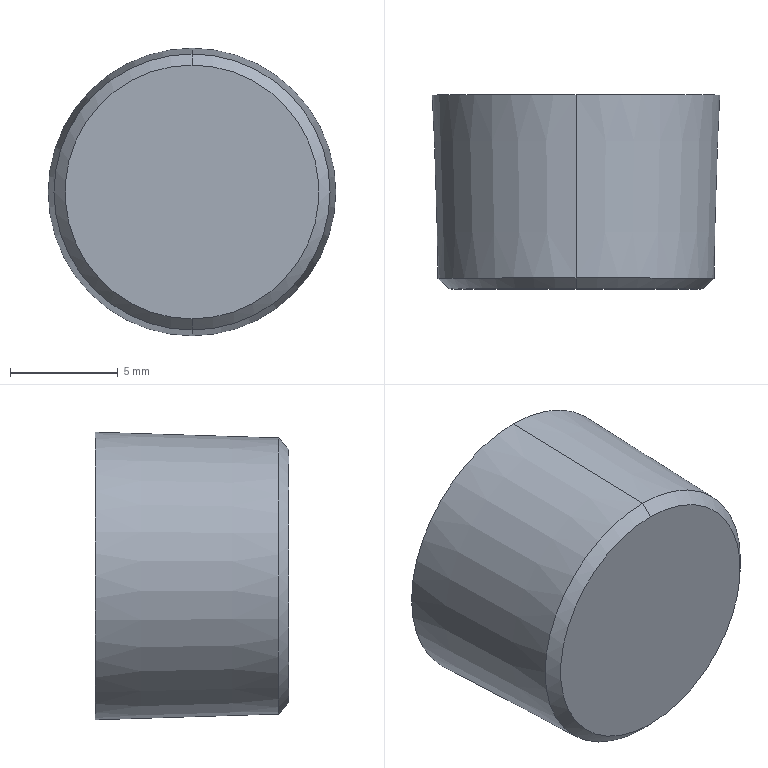Part | SolidWorks | features BaseBody 1 | 1 solid | 23 faces | box 13.344 x 9 x 13.344 mm | volume 1017 mm3 | plane 15 | cone 8
STEP:
#1=CARTESIAN_POINT('',(0.,0.4998,6.407));
#2=VERTEX_POINT('',#1);
#3=CARTESIAN_POINT('',(0.,0.4998,-6.407));
#4=VERTEX_POINT('',#3);
#5=CARTESIAN_POINT('',(0.,0.4998,0.));
#6=DIRECTION('',(0.,1.,0.));
#7=DIRECTION('',(0.,0.,1.));
#8=AXIS2_PLACEMENT_3D('',#5,#6,#7);
#9=CIRCLE('',#8,6.407);
#10=EDGE_CURVE('',#2,#4,#9,.T.);
#11=ORIENTED_EDGE('',*,*,#10,.T.);
#12=CARTESIAN_POINT('',(0.,9.,-6.672));
#13=VERTEX_POINT('',#12);
#14=CARTESIAN_POINT('',(0.,9.,-6.672));
#15=DIRECTION('',(0.,0.9995,-0.0312));
#16=VECTOR('',#15,1000.);
#17=LINE('',#14,#16);
#18=EDGE_CURVE('',#4,#13,#17,.T.);
#19=ORIENTED_EDGE('',*,*,#18,.T.);
#20=CARTESIAN_POINT('',(0.,9.,6.672));
#21=VERTEX_POINT('',#20);
#22=CARTESIAN_POINT('',(0.,9.,0.));
#23=DIRECTION('',(0.,-1.,0.));
#24=DIRECTION('',(0.,0.,1.));
#25=AXIS2_PLACEMENT_3D('',#22,#23,#24);
#26=CIRCLE('',#25,6.672);
#27=EDGE_CURVE('',#13,#21,#26,.T.);
#28=ORIENTED_EDGE('',*,*,#27,.T.);
#29=CARTESIAN_POINT('',(0.,9.,6.672));
#30=DIRECTION('',(0.,0.9995,0.0312));
#31=VECTOR('',#30,1000.);
#32=LINE('',#29,#31);
#33=EDGE_CURVE('',#2,#21,#32,.T.);
#34=ORIENTED_EDGE('',*,*,#33,.F.);
#35=EDGE_LOOP('',(#11,#19,#28,#34));
#36=FACE_OUTER_BOUND('',#35,.T.);
#37=CARTESIAN_POINT('',(0.,9.,0.));
#38=DIRECTION('',(0.,1.,0.));
#39=DIRECTION('',(0.,0.,1.));
#40=AXIS2_PLACEMENT_3D('',#37,#38,#39);
#41=CONICAL_SURFACE('',#40,6.672,0.03121);
#42=ADVANCED_FACE('',(#36),#41,.T.);
#43=CARTESIAN_POINT('',(0.,0.,5.891));
#44=VERTEX_POINT('',#43);
#45=CARTESIAN_POINT('',(0.,0.,-5.891));
#46=VERTEX_POINT('',#45);
#47=CARTESIAN_POINT('',(0.,0.,0.));
#48=DIRECTION('',(0.,1.,0.));
#49=DIRECTION('',(0.,0.,1.));
#50=AXIS2_PLACEMENT_3D('',#47,#48,#49);
#51=CIRCLE('',#50,5.891);
#52=EDGE_CURVE('',#44,#46,#51,.T.);
#53=ORIENTED_EDGE('',*,*,#52,.T.);
#54=CARTESIAN_POINT('',(0.,0.4998,-6.407));
#55=DIRECTION('',(0.,0.696,-0.7181));
#56=VECTOR('',#55,1000.);
#57=LINE('',#54,#56);
#58=EDGE_CURVE('',#46,#4,#57,.T.);
#59=ORIENTED_EDGE('',*,*,#58,.T.);
#60=ORIENTED_EDGE('',*,*,#10,.F.);
#61=CARTESIAN_POINT('',(0.,0.4998,6.407));
#62=DIRECTION('',(0.,0.696,0.7181));
#63=VECTOR('',#62,1000.);
#64=LINE('',#61,#63);
#65=EDGE_CURVE('',#44,#2,#64,.T.);
#66=ORIENTED_EDGE('',*,*,#65,.F.);
#67=EDGE_LOOP('',(#53,#59,#60,#66));
#68=FACE_OUTER_BOUND('',#67,.T.);
#69=CARTESIAN_POINT('',(0.,0.4998,0.));
#70=DIRECTION('',(0.,1.,0.));
#71=DIRECTION('',(0.,0.,1.));
#72=AXIS2_PLACEMENT_3D('',#69,#70,#71);
#73=CONICAL_SURFACE('',#72,6.407,0.801);
#74=ADVANCED_FACE('',(#68),#73,.T.);
#75=CARTESIAN_POINT('',(0.,8.293,-3.));
#76=VERTEX_POINT('',#75);
#77=CARTESIAN_POINT('',(-1.732,8.757,-3.));
#78=VERTEX_POINT('',#77);
#79=CARTESIAN_POINT('',(0.,8.293,-3.));
#80=CARTESIAN_POINT('',(-0.3013,8.293,-3.));
#81=CARTESIAN_POINT('',(-0.5974,8.339,-3.));
#82=CARTESIAN_POINT('',(-1.182,8.505,-3.));
#83=CARTESIAN_POINT('',(-1.461,8.621,-3.));
#84=CARTESIAN_POINT('',(-1.732,8.757,-3.));
#85=B_SPLINE_CURVE_WITH_KNOTS('',3,(#79,#80,#81,#82,#83,#84),.UNSPECIFIED.,.F.,.F.,(4,2,4),(0.001795,0.002687,0.003578),.UNSPECIFIED.);
#86=EDGE_CURVE('',#76,#78,#85,.T.);
#87=ORIENTED_EDGE('',*,*,#86,.F.);
#88=CARTESIAN_POINT('',(0.,9.,-3.707));
#89=VERTEX_POINT('',#88);
#90=CARTESIAN_POINT('',(0.,9.,-3.707));
#91=DIRECTION('',(0.,0.7071,-0.7071));
#92=VECTOR('',#91,1000.);
#93=LINE('',#90,#92);
#94=EDGE_CURVE('',#76,#89,#93,.T.);
#95=ORIENTED_EDGE('',*,*,#94,.T.);
#96=CARTESIAN_POINT('',(0.,9.,3.707));
#97=VERTEX_POINT('',#96);
#98=CARTESIAN_POINT('',(0.,9.,0.));
#99=DIRECTION('',(0.,1.,0.));
#100=DIRECTION('',(0.,0.,1.));
#101=AXIS2_PLACEMENT_3D('',#98,#99,#100);
#102=CIRCLE('',#101,3.707);
#103=EDGE_CURVE('',#89,#97,#102,.T.);
#104=ORIENTED_EDGE('',*,*,#103,.T.);
#105=CARTESIAN_POINT('',(0.,8.293,3.));
#106=VERTEX_POINT('',#105);
#107=CARTESIAN_POINT('',(0.,9.,3.707));
#108=DIRECTION('',(0.,0.7071,0.7071));
#109=VECTOR('',#108,1000.);
#110=LINE('',#107,#109);
#111=EDGE_CURVE('',#106,#97,#110,.T.);
#112=ORIENTED_EDGE('',*,*,#111,.F.);
#113=CARTESIAN_POINT('',(-1.732,8.757,3.));
#114=VERTEX_POINT('',#113);
#115=CARTESIAN_POINT('',(-1.732,8.757,3.));
#116=CARTESIAN_POINT('',(-1.46,8.621,3.));
#117=CARTESIAN_POINT('',(-1.183,8.506,3.));
#118=CARTESIAN_POINT('',(-0.7511,8.382,3.));
#119=CARTESIAN_POINT('',(-0.6047,8.35,3.));
#120=CARTESIAN_POINT('',(-0.3057,8.305,3.));
#121=CARTESIAN_POINT('',(-0.1517,8.293,3.));
#122=CARTESIAN_POINT('',(0.,8.293,3.));
#123=B_SPLINE_CURVE_WITH_KNOTS('',3,(#115,#116,#117,#118,#119,#120,#121,#122),.UNSPECIFIED.,.F.,.F.,(4,2,2,4),(0.,0.0008977,0.001347,0.001795),.UNSPECIFIED.);
#124=EDGE_CURVE('',#114,#106,#123,.T.);
#125=ORIENTED_EDGE('',*,*,#124,.F.);
#126=CARTESIAN_POINT('',(-3.464,8.757,-0.000000032));
#127=VERTEX_POINT('',#126);
#128=CARTESIAN_POINT('',(-3.464,8.757,-0.000000032));
#129=CARTESIAN_POINT('',(-3.329,8.622,0.2344));
#130=CARTESIAN_POINT('',(-3.19,8.507,0.4741));
#131=CARTESIAN_POINT('',(-2.975,8.383,0.8465));
#132=CARTESIAN_POINT('',(-2.902,8.351,0.9728));
#133=CARTESIAN_POINT('',(-2.754,8.305,1.231));
#134=CARTESIAN_POINT('',(-2.677,8.293,1.364));
#135=CARTESIAN_POINT('',(-2.45,8.292,1.756));
#136=CARTESIAN_POINT('',(-2.301,8.338,2.014));
#137=CARTESIAN_POINT('',(-2.008,8.504,2.521));
#138=CARTESIAN_POINT('',(-1.868,8.621,2.764));
#139=CARTESIAN_POINT('',(-1.732,8.757,3.));
#140=B_SPLINE_CURVE_WITH_KNOTS('',3,(#128,#129,#130,#131,#132,#133,#134,#135,#136,#137,#138,#139),.UNSPECIFIED.,.F.,.F.,(4,2,2,2,2,4),(0.,0.0008946,0.001342,0.001789,0.002684,0.003578),.UNSPECIFIED.);
#141=EDGE_CURVE('',#127,#114,#140,.T.);
#142=ORIENTED_EDGE('',*,*,#141,.F.);
#143=CARTESIAN_POINT('',(-1.732,8.757,-3.));
#144=CARTESIAN_POINT('',(-1.867,8.622,-2.766));
#145=CARTESIAN_POINT('',(-2.006,8.507,-2.526));
#146=CARTESIAN_POINT('',(-2.221,8.383,-2.154));
#147=CARTESIAN_POINT('',(-2.294,8.351,-2.027));
#148=CARTESIAN_POINT('',(-2.443,8.305,-1.769));
#149=CARTESIAN_POINT('',(-2.519,8.293,-1.636));
#150=CARTESIAN_POINT('',(-2.746,8.292,-1.244));
#151=CARTESIAN_POINT('',(-2.895,8.338,-0.9862));
#152=CARTESIAN_POINT('',(-3.188,8.504,-0.4785));
#153=CARTESIAN_POINT('',(-3.328,8.621,-0.2358));
#154=CARTESIAN_POINT('',(-3.464,8.757,-0.000000032));
#155=B_SPLINE_CURVE_WITH_KNOTS('',3,(#143,#144,#145,#146,#147,#148,#149,#150,#151,#152,#153,#154),.UNSPECIFIED.,.F.,.F.,(4,2,2,2,2,4),(0.,0.0008946,0.001342,0.001789,0.002684,0.003578),.UNSPECIFIED.);
#156=EDGE_CURVE('',#78,#127,#155,.T.);
#157=ORIENTED_EDGE('',*,*,#156,.F.);
#158=EDGE_LOOP('',(#87,#95,#104,#112,#125,#142,#157));
#159=FACE_OUTER_BOUND('',#158,.T.);
#160=CARTESIAN_POINT('',(0.,9.,0.));
#161=DIRECTION('',(0.,1.,0.));
#162=DIRECTION('',(0.,0.,1.));
#163=AXIS2_PLACEMENT_3D('',#160,#161,#162);
#164=CONICAL_SURFACE('',#163,3.707,0.7854);
#165=ADVANCED_FACE('',(#159),#164,.F.);
#166=CARTESIAN_POINT('',(1.831,3.063,0.));
#167=VERTEX_POINT('',#166);
#168=CARTESIAN_POINT('',(-1.831,3.063,0.));
#169=VERTEX_POINT('',#168);
#170=CARTESIAN_POINT('',(0.,3.063,0.));
#171=DIRECTION('',(0.,1.,0.));
#172=DIRECTION('',(-1.,0.,0.));
#173=AXIS2_PLACEMENT_3D('',#170,#171,#172);
#174=CIRCLE('',#173,1.831);
#175=EDGE_CURVE('',#167,#169,#174,.T.);
#176=ORIENTED_EDGE('',*,*,#175,.F.);
#177=CARTESIAN_POINT('',(3.464,3.5,0.));
#178=VERTEX_POINT('',#177);
#179=CARTESIAN_POINT('',(3.464,3.5,0.));
#180=DIRECTION('',(0.9659,0.2588,0.));
#181=VECTOR('',#180,1000.);
#182=LINE('',#179,#181);
#183=EDGE_CURVE('',#167,#178,#182,.T.);
#184=ORIENTED_EDGE('',*,*,#183,.T.);
#185=CARTESIAN_POINT('',(1.732,3.5,-3.));
#186=VERTEX_POINT('',#185);
#187=CARTESIAN_POINT('',(0.,3.5,0.));
#188=DIRECTION('',(0.,-1.,0.));
#189=DIRECTION('',(-1.,0.,0.));
#190=AXIS2_PLACEMENT_3D('',#187,#188,#189);
#191=CIRCLE('',#190,3.464);
#192=EDGE_CURVE('',#186,#178,#191,.T.);
#193=ORIENTED_EDGE('',*,*,#192,.F.);
#194=CARTESIAN_POINT('',(-1.732,3.5,-3.));
#195=VERTEX_POINT('',#194);
#196=CARTESIAN_POINT('',(0.,3.5,0.));
#197=DIRECTION('',(0.,-1.,0.));
#198=DIRECTION('',(-1.,0.,0.));
#199=AXIS2_PLACEMENT_3D('',#196,#197,#198);
#200=CIRCLE('',#199,3.464);
#201=EDGE_CURVE('',#195,#186,#200,.T.);
#202=ORIENTED_EDGE('',*,*,#201,.F.);
#203=CARTESIAN_POINT('',(-3.464,3.5,0.));
#204=VERTEX_POINT('',#203);
#205=CARTESIAN_POINT('',(0.,3.5,0.));
#206=DIRECTION('',(0.,-1.,0.));
#207=DIRECTION('',(-1.,0.,0.));
#208=AXIS2_PLACEMENT_3D('',#205,#206,#207);
#209=CIRCLE('',#208,3.464);
#210=EDGE_CURVE('',#204,#195,#209,.T.);
#211=ORIENTED_EDGE('',*,*,#210,.F.);
#212=CARTESIAN_POINT('',(-3.464,3.5,0.));
#213=DIRECTION('',(-0.9659,0.2588,0.));
#214=VECTOR('',#213,1000.);
#215=LINE('',#212,#214);
#216=EDGE_CURVE('',#169,#204,#215,.T.);
#217=ORIENTED_EDGE('',*,*,#216,.F.);
#218=EDGE_LOOP('',(#176,#184,#193,#202,#211,#217));
#219=FACE_OUTER_BOUND('',#218,.T.);
#220=CARTESIAN_POINT('',(0.,3.5,0.));
#221=DIRECTION('',(0.,1.,0.));
#222=DIRECTION('',(-1.,0.,0.));
#223=AXIS2_PLACEMENT_3D('',#220,#221,#222);
#224=CONICAL_SURFACE('',#223,3.464,1.309);
#225=ADVANCED_FACE('',(#219),#224,.F.);
#226=ORIENTED_EDGE('',*,*,#18,.F.);
#227=CARTESIAN_POINT('',(0.,0.4998,0.));
#228=DIRECTION('',(0.,1.,0.));
#229=DIRECTION('',(0.,0.,1.));
#230=AXIS2_PLACEMENT_3D('',#227,#228,#229);
#231=CIRCLE('',#230,6.407);
#232=EDGE_CURVE('',#4,#2,#231,.T.);
#233=ORIENTED_EDGE('',*,*,#232,.T.);
#234=ORIENTED_EDGE('',*,*,#33,.T.);
#235=CARTESIAN_POINT('',(0.,9.,0.));
#236=DIRECTION('',(0.,-1.,0.));
#237=DIRECTION('',(0.,0.,1.));
#238=AXIS2_PLACEMENT_3D('',#235,#236,#237);
#239=CIRCLE('',#238,6.672);
#240=EDGE_CURVE('',#21,#13,#239,.T.);
#241=ORIENTED_EDGE('',*,*,#240,.T.);
#242=EDGE_LOOP('',(#226,#233,#234,#241));
#243=FACE_OUTER_BOUND('',#242,.T.);
#244=CARTESIAN_POINT('',(0.,9.,0.));
#245=DIRECTION('',(0.,1.,0.));
#246=DIRECTION('',(0.,0.,1.));
#247=AXIS2_PLACEMENT_3D('',#244,#245,#246);
#248=CONICAL_SURFACE('',#247,6.672,0.03121);
#249=ADVANCED_FACE('',(#243),#248,.T.);
#250=CARTESIAN_POINT('',(0.,9.,0.));
#251=DIRECTION('',(0.,1.,0.));
#252=DIRECTION('',(0.,0.,1.));
#253=AXIS2_PLACEMENT_3D('',#250,#251,#252);
#254=CIRCLE('',#253,3.707);
#255=EDGE_CURVE('',#97,#89,#254,.T.);
#256=ORIENTED_EDGE('',*,*,#255,.F.);
#257=ORIENTED_EDGE('',*,*,#103,.F.);
#258=EDGE_LOOP('',(#256,#257));
#259=FACE_BOUND('',#258,.T.);
#260=ORIENTED_EDGE('',*,*,#240,.F.);
#261=ORIENTED_EDGE('',*,*,#27,.F.);
#262=EDGE_LOOP('',(#260,#261));
#263=FACE_OUTER_BOUND('',#262,.T.);
#264=CARTESIAN_POINT('',(3.707,9.,0.));
#265=DIRECTION('',(0.,-1.,0.));
#266=DIRECTION('',(0.,0.,-1.));
#267=AXIS2_PLACEMENT_3D('',#264,#265,#266);
#268=PLANE('',#267);
#269=ADVANCED_FACE('',(#259,#263),#268,.F.);
#270=ORIENTED_EDGE('',*,*,#58,.F.);
#271=CARTESIAN_POINT('',(0.,0.,0.));
#272=DIRECTION('',(0.,1.,0.));
#273=DIRECTION('',(0.,0.,1.));
#274=AXIS2_PLACEMENT_3D('',#271,#272,#273);
#275=CIRCLE('',#274,5.891);
#276=EDGE_CURVE('',#46,#44,#275,.T.);
#277=ORIENTED_EDGE('',*,*,#276,.T.);
#278=ORIENTED_EDGE('',*,*,#65,.T.);
#279=ORIENTED_EDGE('',*,*,#232,.F.);
#280=EDGE_LOOP('',(#270,#277,#278,#279));
#281=FACE_OUTER_BOUND('',#280,.T.);
#282=CARTESIAN_POINT('',(0.,0.4998,0.));
#283=DIRECTION('',(0.,1.,0.));
#284=DIRECTION('',(0.,0.,1.));
#285=AXIS2_PLACEMENT_3D('',#282,#283,#284);
#286=CONICAL_SURFACE('',#285,6.407,0.801);
#287=ADVANCED_FACE('',(#281),#286,.T.);
#288=ORIENTED_EDGE('',*,*,#94,.F.);
#289=CARTESIAN_POINT('',(1.732,8.757,-3.));
#290=VERTEX_POINT('',#289);
#291=CARTESIAN_POINT('',(1.732,8.757,-3.));
#292=CARTESIAN_POINT('',(1.46,8.621,-3.));
#293=CARTESIAN_POINT('',(1.183,8.506,-3.));
#294=CARTESIAN_POINT('',(0.7511,8.382,-3.));
#295=CARTESIAN_POINT('',(0.6047,8.35,-3.));
#296=CARTESIAN_POINT('',(0.3057,8.305,-3.));
#297=CARTESIAN_POINT('',(0.1517,8.293,-3.));
#298=CARTESIAN_POINT('',(0.,8.293,-3.));
#299=B_SPLINE_CURVE_WITH_KNOTS('',3,(#291,#292,#293,#294,#295,#296,#297,#298),.UNSPECIFIED.,.F.,.F.,(4,2,2,4),(0.,0.0008977,0.001347,0.001795),.UNSPECIFIED.);
#300=EDGE_CURVE('',#290,#76,#299,.T.);
#301=ORIENTED_EDGE('',*,*,#300,.F.);
#302=CARTESIAN_POINT('',(3.464,8.757,-0.000000012));
#303=VERTEX_POINT('',#302);
#304=CARTESIAN_POINT('',(3.464,8.757,-0.000000012));
#305=CARTESIAN_POINT('',(3.329,8.622,-0.2344));
#306=CARTESIAN_POINT('',(3.19,8.507,-0.4741));
#307=CARTESIAN_POINT('',(2.975,8.383,-0.8465));
#308=CARTESIAN_POINT('',(2.902,8.351,-0.9728));
#309=CARTESIAN_POINT('',(2.754,8.305,-1.231));
#310=CARTESIAN_POINT('',(2.677,8.293,-1.364));
#311=CARTESIAN_POINT('',(2.45,8.292,-1.756));
#312=CARTESIAN_POINT('',(2.301,8.338,-2.014));
#313=CARTESIAN_POINT('',(2.008,8.504,-2.521));
#314=CARTESIAN_POINT('',(1.868,8.621,-2.764));
#315=CARTESIAN_POINT('',(1.732,8.757,-3.));
#316=B_SPLINE_CURVE_WITH_KNOTS('',3,(#304,#305,#306,#307,#308,#309,#310,#311,#312,#313,#314,#315),.UNSPECIFIED.,.F.,.F.,(4,2,2,2,2,4),(0.,0.0008946,0.001342,0.001789,0.002684,0.003578),.UNSPECIFIED.);
#317=EDGE_CURVE('',#303,#290,#316,.T.);
#318=ORIENTED_EDGE('',*,*,#317,.F.);
#319=CARTESIAN_POINT('',(1.732,8.757,3.));
#320=VERTEX_POINT('',#319);
#321=CARTESIAN_POINT('',(1.732,8.757,3.));
#322=CARTESIAN_POINT('',(1.867,8.622,2.766));
#323=CARTESIAN_POINT('',(2.006,8.507,2.526));
#324=CARTESIAN_POINT('',(2.221,8.383,2.154));
#325=CARTESIAN_POINT('',(2.294,8.351,2.027));
#326=CARTESIAN_POINT('',(2.443,8.305,1.769));
#327=CARTESIAN_POINT('',(2.519,8.293,1.636));
#328=CARTESIAN_POINT('',(2.746,8.292,1.244));
#329=CARTESIAN_POINT('',(2.895,8.338,0.9862));
#330=CARTESIAN_POINT('',(3.188,8.504,0.4785));
#331=CARTESIAN_POINT('',(3.328,8.621,0.2358));
#332=CARTESIAN_POINT('',(3.464,8.757,-0.000000012));
#333=B_SPLINE_CURVE_WITH_KNOTS('',3,(#321,#322,#323,#324,#325,#326,#327,#328,#329,#330,#331,#332),.UNSPECIFIED.,.F.,.F.,(4,2,2,2,2,4),(0.,0.0008946,0.001342,0.001789,0.002684,0.003578),.UNSPECIFIED.);
#334=EDGE_CURVE('',#320,#303,#333,.T.);
#335=ORIENTED_EDGE('',*,*,#334,.F.);
#336=CARTESIAN_POINT('',(0.,8.293,3.));
#337=CARTESIAN_POINT('',(0.3013,8.293,3.));
#338=CARTESIAN_POINT('',(0.5974,8.339,3.));
#339=CARTESIAN_POINT('',(1.182,8.505,3.));
#340=CARTESIAN_POINT('',(1.461,8.621,3.));
#341=CARTESIAN_POINT('',(1.732,8.757,3.));
#342=B_SPLINE_CURVE_WITH_KNOTS('',3,(#336,#337,#338,#339,#340,#341),.UNSPECIFIED.,.F.,.F.,(4,2,4),(0.001795,0.002687,0.003578),.UNSPECIFIED.);
#343=EDGE_CURVE('',#106,#320,#342,.T.);
#344=ORIENTED_EDGE('',*,*,#343,.F.);
#345=ORIENTED_EDGE('',*,*,#111,.T.);
#346=ORIENTED_EDGE('',*,*,#255,.T.);
#347=EDGE_LOOP('',(#288,#301,#318,#335,#344,#345,#346));
#348=FACE_OUTER_BOUND('',#347,.T.);
#349=CARTESIAN_POINT('',(0.,9.,0.));
#350=DIRECTION('',(0.,1.,0.));
#351=DIRECTION('',(0.,0.,1.));
#352=AXIS2_PLACEMENT_3D('',#349,#350,#351);
#353=CONICAL_SURFACE('',#352,3.707,0.7854);
#354=ADVANCED_FACE('',(#348),#353,.F.);
#355=ORIENTED_EDGE('',*,*,#52,.F.);
#356=ORIENTED_EDGE('',*,*,#276,.F.);
#357=EDGE_LOOP('',(#355,#356));
#358=FACE_OUTER_BOUND('',#357,.T.);
#359=CARTESIAN_POINT('',(5.891,0.,0.));
#360=DIRECTION('',(0.,1.,0.));
#361=DIRECTION('',(0.,0.,1.));
#362=AXIS2_PLACEMENT_3D('',#359,#360,#361);
#363=PLANE('',#362);
#364=ADVANCED_FACE('',(#358),#363,.F.);
#365=CARTESIAN_POINT('',(1.732,3.5,3.));
#366=VERTEX_POINT('',#365);
#367=CARTESIAN_POINT('',(1.732,3.5,3.));
#368=DIRECTION('',(0.,-1.,0.));
#369=VECTOR('',#368,1000.);
#370=LINE('',#367,#369);
#371=EDGE_CURVE('',#320,#366,#370,.T.);
#372=ORIENTED_EDGE('',*,*,#371,.F.);
#373=ORIENTED_EDGE('',*,*,#334,.T.);
#374=CARTESIAN_POINT('',(3.464,3.5,0.));
#375=DIRECTION('',(0.,1.,0.));
#376=VECTOR('',#375,1000.);
#377=LINE('',#374,#376);
#378=EDGE_CURVE('',#178,#303,#377,.T.);
#379=ORIENTED_EDGE('',*,*,#378,.F.);
#380=CARTESIAN_POINT('',(1.732,3.5,3.));
#381=DIRECTION('',(0.5,0.,-0.866));
#382=VECTOR('',#381,1000.);
#383=LINE('',#380,#382);
#384=EDGE_CURVE('',#366,#178,#383,.T.);
#385=ORIENTED_EDGE('',*,*,#384,.F.);
#386=EDGE_LOOP('',(#372,#373,#379,#385));
#387=FACE_OUTER_BOUND('',#386,.T.);
#388=CARTESIAN_POINT('',(1.732,3.5,3.));
#389=DIRECTION('',(0.866,0.,0.5));
#390=DIRECTION('',(0.5,0.,-0.866));
#391=AXIS2_PLACEMENT_3D('',#388,#389,#390);
#392=PLANE('',#391);
#393=ADVANCED_FACE('',(#387),#392,.F.);
#394=CARTESIAN_POINT('',(-1.732,3.5,3.));
#395=VERTEX_POINT('',#394);
#396=CARTESIAN_POINT('',(-1.732,3.5,3.));
#397=DIRECTION('',(0.,-1.,0.));
#398=VECTOR('',#397,1000.);
#399=LINE('',#396,#398);
#400=EDGE_CURVE('',#114,#395,#399,.T.);
#401=ORIENTED_EDGE('',*,*,#400,.F.);
#402=ORIENTED_EDGE('',*,*,#124,.T.);
#403=ORIENTED_EDGE('',*,*,#343,.T.);
#404=ORIENTED_EDGE('',*,*,#371,.T.);
#405=CARTESIAN_POINT('',(-1.732,3.5,3.));
#406=DIRECTION('',(1.,0.,0.));
#407=VECTOR('',#406,1000.);
#408=LINE('',#405,#407);
#409=EDGE_CURVE('',#395,#366,#408,.T.);
#410=ORIENTED_EDGE('',*,*,#409,.F.);
#411=EDGE_LOOP('',(#401,#402,#403,#404,#410));
#412=FACE_OUTER_BOUND('',#411,.T.);
#413=CARTESIAN_POINT('',(-1.732,3.5,3.));
#414=DIRECTION('',(0.,0.,1.));
#415=DIRECTION('',(1.,0.,0.));
#416=AXIS2_PLACEMENT_3D('',#413,#414,#415);
#417=PLANE('',#416);
#418=ADVANCED_FACE('',(#412),#417,.F.);
#419=CARTESIAN_POINT('',(-3.464,3.5,0.));
#420=DIRECTION('',(0.,-1.,0.));
#421=VECTOR('',#420,1000.);
#422=LINE('',#419,#421);
#423=EDGE_CURVE('',#127,#204,#422,.T.);
#424=ORIENTED_EDGE('',*,*,#423,.F.);
#425=ORIENTED_EDGE('',*,*,#141,.T.);
#426=ORIENTED_EDGE('',*,*,#400,.T.);
#427=CARTESIAN_POINT('',(-3.464,3.5,0.));
#428=DIRECTION('',(0.5,0.,0.866));
#429=VECTOR('',#428,1000.);
#430=LINE('',#427,#429);
#431=EDGE_CURVE('',#204,#395,#430,.T.);
#432=ORIENTED_EDGE('',*,*,#431,.F.);
#433=EDGE_LOOP('',(#424,#425,#426,#432));
#434=FACE_OUTER_BOUND('',#433,.T.);
#435=CARTESIAN_POINT('',(-3.464,3.5,0.));
#436=DIRECTION('',(-0.866,0.,0.5));
#437=DIRECTION('',(0.5,0.,0.866));
#438=AXIS2_PLACEMENT_3D('',#435,#436,#437);
#439=PLANE('',#438);
#440=ADVANCED_FACE('',(#434),#439,.F.);
#441=CARTESIAN_POINT('',(-1.732,3.5,-3.));
#442=DIRECTION('',(0.,-1.,0.));
#443=VECTOR('',#442,1000.);
#444=LINE('',#441,#443);
#445=EDGE_CURVE('',#78,#195,#444,.T.);
#446=ORIENTED_EDGE('',*,*,#445,.F.);
#447=ORIENTED_EDGE('',*,*,#156,.T.);
#448=ORIENTED_EDGE('',*,*,#423,.T.);
#449=CARTESIAN_POINT('',(-1.732,3.5,-3.));
#450=DIRECTION('',(-0.5,0.,0.866));
#451=VECTOR('',#450,1000.);
#452=LINE('',#449,#451);
#453=EDGE_CURVE('',#195,#204,#452,.T.);
#454=ORIENTED_EDGE('',*,*,#453,.F.);
#455=EDGE_LOOP('',(#446,#447,#448,#454));
#456=FACE_OUTER_BOUND('',#455,.T.);
#457=CARTESIAN_POINT('',(-1.732,3.5,-3.));
#458=DIRECTION('',(-0.866,0.,-0.5));
#459=DIRECTION('',(-0.5,0.,0.866));
#460=AXIS2_PLACEMENT_3D('',#457,#458,#459);
#461=PLANE('',#460);
#462=ADVANCED_FACE('',(#456),#461,.F.);
#463=CARTESIAN_POINT('',(1.732,3.5,-3.));
#464=DIRECTION('',(0.,-1.,0.));
#465=VECTOR('',#464,1000.);
#466=LINE('',#463,#465);
#467=EDGE_CURVE('',#290,#186,#466,.T.);
#468=ORIENTED_EDGE('',*,*,#467,.F.);
#469=ORIENTED_EDGE('',*,*,#300,.T.);
#470=ORIENTED_EDGE('',*,*,#86,.T.);
#471=ORIENTED_EDGE('',*,*,#445,.T.);
#472=CARTESIAN_POINT('',(1.732,3.5,-3.));
#473=DIRECTION('',(-1.,0.,0.));
#474=VECTOR('',#473,1000.);
#475=LINE('',#472,#474);
#476=EDGE_CURVE('',#186,#195,#475,.T.);
#477=ORIENTED_EDGE('',*,*,#476,.F.);
#478=EDGE_LOOP('',(#468,#469,#470,#471,#477));
#479=FACE_OUTER_BOUND('',#478,.T.);
#480=CARTESIAN_POINT('',(1.732,3.5,-3.));
#481=DIRECTION('',(0.,0.,-1.));
#482=DIRECTION('',(-1.,0.,0.));
#483=AXIS2_PLACEMENT_3D('',#480,#481,#482);
#484=PLANE('',#483);
#485=ADVANCED_FACE('',(#479),#484,.F.);
#486=ORIENTED_EDGE('',*,*,#378,.T.);
#487=ORIENTED_EDGE('',*,*,#317,.T.);
#488=ORIENTED_EDGE('',*,*,#467,.T.);
#489=CARTESIAN_POINT('',(3.464,3.5,0.));
#490=DIRECTION('',(-0.5,0.,-0.866));
#491=VECTOR('',#490,1000.);
#492=LINE('',#489,#491);
#493=EDGE_CURVE('',#178,#186,#492,.T.);
#494=ORIENTED_EDGE('',*,*,#493,.F.);
#495=EDGE_LOOP('',(#486,#487,#488,#494));
#496=FACE_OUTER_BOUND('',#495,.T.);
#497=CARTESIAN_POINT('',(3.464,3.5,0.));
#498=DIRECTION('',(0.866,0.,-0.5));
#499=DIRECTION('',(-0.5,0.,-0.866));
#500=AXIS2_PLACEMENT_3D('',#497,#498,#499);
#501=PLANE('',#500);
#502=ADVANCED_FACE('',(#496),#501,.F.);
#503=ORIENTED_EDGE('',*,*,#384,.T.);
#504=CARTESIAN_POINT('',(0.,3.5,0.));
#505=DIRECTION('',(0.,-1.,0.));
#506=DIRECTION('',(-1.,0.,0.));
#507=AXIS2_PLACEMENT_3D('',#504,#505,#506);
#508=CIRCLE('',#507,3.464);
#509=EDGE_CURVE('',#178,#366,#508,.T.);
#510=ORIENTED_EDGE('',*,*,#509,.T.);
#511=EDGE_LOOP('',(#503,#510));
#512=FACE_OUTER_BOUND('',#511,.T.);
#513=CARTESIAN_POINT('',(0.,3.5,0.));
#514=DIRECTION('',(0.,-1.,0.));
#515=DIRECTION('',(1.,0.,0.));
#516=AXIS2_PLACEMENT_3D('',#513,#514,#515);
#517=PLANE('',#516);
#518=ADVANCED_FACE('',(#512),#517,.T.);
#519=ORIENTED_EDGE('',*,*,#409,.T.);
#520=CARTESIAN_POINT('',(0.,3.5,0.));
#521=DIRECTION('',(0.,-1.,0.));
#522=DIRECTION('',(-1.,0.,0.));
#523=AXIS2_PLACEMENT_3D('',#520,#521,#522);
#524=CIRCLE('',#523,3.464);
#525=EDGE_CURVE('',#366,#395,#524,.T.);
#526=ORIENTED_EDGE('',*,*,#525,.T.);
#527=EDGE_LOOP('',(#519,#526));
#528=FACE_OUTER_BOUND('',#527,.T.);
#529=CARTESIAN_POINT('',(0.,3.5,0.));
#530=DIRECTION('',(0.,-1.,0.));
#531=DIRECTION('',(1.,0.,0.));
#532=AXIS2_PLACEMENT_3D('',#529,#530,#531);
#533=PLANE('',#532);
#534=ADVANCED_FACE('',(#528),#533,.T.);
#535=ORIENTED_EDGE('',*,*,#431,.T.);
#536=CARTESIAN_POINT('',(0.,3.5,0.));
#537=DIRECTION('',(0.,-1.,0.));
#538=DIRECTION('',(-1.,0.,0.));
#539=AXIS2_PLACEMENT_3D('',#536,#537,#538);
#540=CIRCLE('',#539,3.464);
#541=EDGE_CURVE('',#395,#204,#540,.T.);
#542=ORIENTED_EDGE('',*,*,#541,.T.);
#543=EDGE_LOOP('',(#535,#542));
#544=FACE_OUTER_BOUND('',#543,.T.);
#545=CARTESIAN_POINT('',(0.,3.5,0.));
#546=DIRECTION('',(0.,-1.,0.));
#547=DIRECTION('',(1.,0.,0.));
#548=AXIS2_PLACEMENT_3D('',#545,#546,#547);
#549=PLANE('',#548);
#550=ADVANCED_FACE('',(#544),#549,.T.);
#551=ORIENTED_EDGE('',*,*,#453,.T.);
#552=ORIENTED_EDGE('',*,*,#210,.T.);
#553=EDGE_LOOP('',(#551,#552));
#554=FACE_OUTER_BOUND('',#553,.T.);
#555=CARTESIAN_POINT('',(0.,3.5,0.));
#556=DIRECTION('',(0.,-1.,0.));
#557=DIRECTION('',(1.,0.,0.));
#558=AXIS2_PLACEMENT_3D('',#555,#556,#557);
#559=PLANE('',#558);
#560=ADVANCED_FACE('',(#554),#559,.T.);
#561=ORIENTED_EDGE('',*,*,#476,.T.);
#562=ORIENTED_EDGE('',*,*,#201,.T.);
#563=EDGE_LOOP('',(#561,#562));
#564=FACE_OUTER_BOUND('',#563,.T.);
#565=CARTESIAN_POINT('',(0.,3.5,0.));
#566=DIRECTION('',(0.,-1.,0.));
#567=DIRECTION('',(1.,0.,0.));
#568=AXIS2_PLACEMENT_3D('',#565,#566,#567);
#569=PLANE('',#568);
#570=ADVANCED_FACE('',(#564),#569,.T.);
#571=ORIENTED_EDGE('',*,*,#493,.T.);
#572=ORIENTED_EDGE('',*,*,#192,.T.);
#573=EDGE_LOOP('',(#571,#572));
#574=FACE_OUTER_BOUND('',#573,.T.);
#575=CARTESIAN_POINT('',(0.,3.5,0.));
#576=DIRECTION('',(0.,-1.,0.));
#577=DIRECTION('',(1.,0.,0.));
#578=AXIS2_PLACEMENT_3D('',#575,#576,#577);
#579=PLANE('',#578);
#580=ADVANCED_FACE('',(#574),#579,.T.);
#581=ORIENTED_EDGE('',*,*,#183,.F.);
#582=CARTESIAN_POINT('',(0.,3.063,0.));
#583=DIRECTION('',(0.,1.,0.));
#584=DIRECTION('',(-1.,0.,0.));
#585=AXIS2_PLACEMENT_3D('',#582,#583,#584);
#586=CIRCLE('',#585,1.831);
#587=EDGE_CURVE('',#169,#167,#586,.T.);
#588=ORIENTED_EDGE('',*,*,#587,.F.);
#589=ORIENTED_EDGE('',*,*,#216,.T.);
#590=ORIENTED_EDGE('',*,*,#541,.F.);
#591=ORIENTED_EDGE('',*,*,#525,.F.);
#592=ORIENTED_EDGE('',*,*,#509,.F.);
#593=EDGE_LOOP('',(#581,#588,#589,#590,#591,#592));
#594=FACE_OUTER_BOUND('',#593,.T.);
#595=CARTESIAN_POINT('',(0.,3.5,0.));
#596=DIRECTION('',(0.,1.,0.));
#597=DIRECTION('',(-1.,0.,0.));
#598=AXIS2_PLACEMENT_3D('',#595,#596,#597);
#599=CONICAL_SURFACE('',#598,3.464,1.309);
#600=ADVANCED_FACE('',(#594),#599,.F.);
#601=ORIENTED_EDGE('',*,*,#587,.T.);
#602=ORIENTED_EDGE('',*,*,#175,.T.);
#603=EDGE_LOOP('',(#601,#602));
#604=FACE_OUTER_BOUND('',#603,.T.);
#605=CARTESIAN_POINT('',(1.831,3.063,0.));
#606=DIRECTION('',(0.,1.,0.));
#607=DIRECTION('',(-1.,0.,0.));
#608=AXIS2_PLACEMENT_3D('',#605,#606,#607);
#609=PLANE('',#608);
#610=ADVANCED_FACE('',(#604),#609,.T.);
#611=CLOSED_SHELL('',(#42,#74,#165,#225,#249,#269,#287,#354,#364,#393,#418,#440,#462,#485,#502,#518,#534,#550,#560,#570,#580,#600,#610));
#612=MANIFOLD_SOLID_BREP('',#611);
#613=CARTESIAN_POINT('',(0.,0.,0.));
#614=DIRECTION('',(0.,0.,1.));
#615=DIRECTION('',(1.,0.,0.));
#616=AXIS2_PLACEMENT_3D('',#613,#614,#615);
#617=(LENGTH_UNIT()NAMED_UNIT(*)SI_UNIT(.MILLI.,.METRE.));
#618=UNCERTAINTY_MEASURE_WITH_UNIT(LENGTH_MEASURE(0.00001),#617,'','');
#619=(NAMED_UNIT(*)PLANE_ANGLE_UNIT()SI_UNIT($,.RADIAN.));
#620=(NAMED_UNIT(*)SI_UNIT($,.STERADIAN.)SOLID_ANGLE_UNIT());
#621=(GEOMETRIC_REPRESENTATION_CONTEXT(3)GLOBAL_UNCERTAINTY_ASSIGNED_CONTEXT((#618))GLOBAL_UNIT_ASSIGNED_CONTEXT((#617,#619,#620))REPRESENTATION_CONTEXT('',''));
#622=ADVANCED_BREP_SHAPE_REPRESENTATION('',(#612,#616),#621);